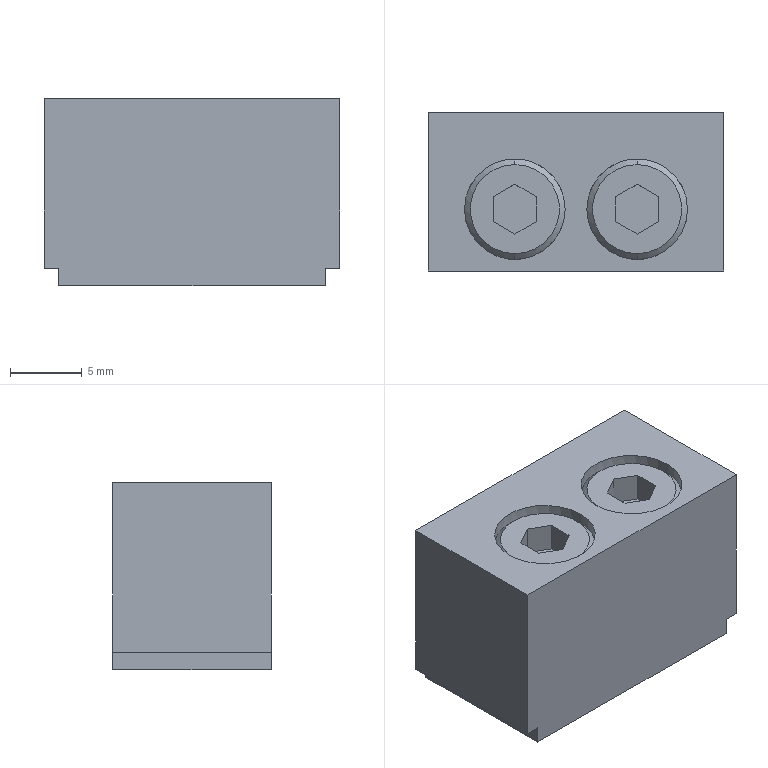Part | SolidWorks | features RefAxis 6, ICE 3, 3DProfileFeature 2, HoleWzd 2, Revolution 2, Extrusion 1 | 1 solid | 34 faces | box 20.5 x 11 x 13 mm | volume 2840 mm3 | plane 26 | cone 4 | cylinder 4 | commonest cylinder face diameters 7 x4
STEP:
#1=CARTESIAN_POINT('',(14.5,1.2,-0.4));
#2=VERTEX_POINT('',#1);
#3=CARTESIAN_POINT('',(14.5,7.4,-0.4));
#4=VERTEX_POINT('',#3);
#5=CARTESIAN_POINT('',(14.5,4.3,-0.4));
#6=DIRECTION('',(0.,0.,1.));
#7=DIRECTION('',(0.,-1.,0.));
#8=AXIS2_PLACEMENT_3D('',#5,#6,#7);
#9=CIRCLE('',#8,3.1);
#10=EDGE_CURVE('',#2,#4,#9,.T.);
#11=ORIENTED_EDGE('',*,*,#10,.F.);
#12=CARTESIAN_POINT('',(14.5,0.8,-0.8));
#13=VERTEX_POINT('',#12);
#14=CARTESIAN_POINT('',(14.5,0.8,-0.8));
#15=DIRECTION('',(0.,-0.7071,-0.7071));
#16=VECTOR('',#15,1000.);
#17=LINE('',#14,#16);
#18=EDGE_CURVE('',#2,#13,#17,.T.);
#19=ORIENTED_EDGE('',*,*,#18,.T.);
#20=CARTESIAN_POINT('',(18.,4.3,-0.8));
#21=VERTEX_POINT('',#20);
#22=CARTESIAN_POINT('',(14.5,4.3,-0.8));
#23=DIRECTION('',(0.,0.,1.));
#24=DIRECTION('',(0.,1.,0.));
#25=AXIS2_PLACEMENT_3D('',#22,#23,#24);
#26=CIRCLE('',#25,3.5);
#27=EDGE_CURVE('',#13,#21,#26,.T.);
#28=ORIENTED_EDGE('',*,*,#27,.T.);
#29=CARTESIAN_POINT('',(14.5,7.8,-0.8));
#30=VERTEX_POINT('',#29);
#31=CARTESIAN_POINT('',(14.5,4.3,-0.8));
#32=DIRECTION('',(0.,0.,1.));
#33=DIRECTION('',(0.,1.,0.));
#34=AXIS2_PLACEMENT_3D('',#31,#32,#33);
#35=CIRCLE('',#34,3.5);
#36=EDGE_CURVE('',#21,#30,#35,.T.);
#37=ORIENTED_EDGE('',*,*,#36,.T.);
#38=CARTESIAN_POINT('',(14.5,7.8,-0.8));
#39=DIRECTION('',(0.,0.7071,-0.7071));
#40=VECTOR('',#39,1000.);
#41=LINE('',#38,#40);
#42=EDGE_CURVE('',#4,#30,#41,.T.);
#43=ORIENTED_EDGE('',*,*,#42,.F.);
#44=EDGE_LOOP('',(#11,#19,#28,#37,#43));
#45=FACE_OUTER_BOUND('',#44,.T.);
#46=CARTESIAN_POINT('',(14.5,4.3,-0.8));
#47=DIRECTION('',(0.,0.,-1.));
#48=DIRECTION('',(0.,1.,0.));
#49=AXIS2_PLACEMENT_3D('',#46,#47,#48);
#50=CONICAL_SURFACE('',#49,3.5,0.7854);
#51=ADVANCED_FACE('',(#45),#50,.T.);
#52=CARTESIAN_POINT('',(6.,1.2,-0.4));
#53=VERTEX_POINT('',#52);
#54=CARTESIAN_POINT('',(6.,7.4,-0.4));
#55=VERTEX_POINT('',#54);
#56=CARTESIAN_POINT('',(6.,4.3,-0.4));
#57=DIRECTION('',(0.,0.,1.));
#58=DIRECTION('',(0.,-1.,0.));
#59=AXIS2_PLACEMENT_3D('',#56,#57,#58);
#60=CIRCLE('',#59,3.1);
#61=EDGE_CURVE('',#53,#55,#60,.T.);
#62=ORIENTED_EDGE('',*,*,#61,.F.);
#63=CARTESIAN_POINT('',(6.,0.8,-0.8));
#64=VERTEX_POINT('',#63);
#65=CARTESIAN_POINT('',(6.,0.8,-0.8));
#66=DIRECTION('',(0.,-0.7071,-0.7071));
#67=VECTOR('',#66,1000.);
#68=LINE('',#65,#67);
#69=EDGE_CURVE('',#53,#64,#68,.T.);
#70=ORIENTED_EDGE('',*,*,#69,.T.);
#71=CARTESIAN_POINT('',(9.5,4.3,-0.8));
#72=VERTEX_POINT('',#71);
#73=CARTESIAN_POINT('',(6.,4.3,-0.8));
#74=DIRECTION('',(0.,0.,1.));
#75=DIRECTION('',(0.,1.,0.));
#76=AXIS2_PLACEMENT_3D('',#73,#74,#75);
#77=CIRCLE('',#76,3.5);
#78=EDGE_CURVE('',#64,#72,#77,.T.);
#79=ORIENTED_EDGE('',*,*,#78,.T.);
#80=CARTESIAN_POINT('',(6.,7.8,-0.8));
#81=VERTEX_POINT('',#80);
#82=CARTESIAN_POINT('',(6.,4.3,-0.8));
#83=DIRECTION('',(0.,0.,1.));
#84=DIRECTION('',(0.,1.,0.));
#85=AXIS2_PLACEMENT_3D('',#82,#83,#84);
#86=CIRCLE('',#85,3.5);
#87=EDGE_CURVE('',#72,#81,#86,.T.);
#88=ORIENTED_EDGE('',*,*,#87,.T.);
#89=CARTESIAN_POINT('',(6.,7.8,-0.8));
#90=DIRECTION('',(0.,0.7071,-0.7071));
#91=VECTOR('',#90,1000.);
#92=LINE('',#89,#91);
#93=EDGE_CURVE('',#55,#81,#92,.T.);
#94=ORIENTED_EDGE('',*,*,#93,.F.);
#95=EDGE_LOOP('',(#62,#70,#79,#88,#94));
#96=FACE_OUTER_BOUND('',#95,.T.);
#97=CARTESIAN_POINT('',(6.,4.3,-0.8));
#98=DIRECTION('',(0.,0.,-1.));
#99=DIRECTION('',(0.,1.,0.));
#100=AXIS2_PLACEMENT_3D('',#97,#98,#99);
#101=CONICAL_SURFACE('',#100,3.5,0.7854);
#102=ADVANCED_FACE('',(#96),#101,.T.);
#103=CARTESIAN_POINT('',(2.5,4.3,-0.8));
#104=VERTEX_POINT('',#103);
#105=CARTESIAN_POINT('',(6.,4.3,-0.8));
#106=DIRECTION('',(0.,0.,1.));
#107=DIRECTION('',(0.,1.,0.));
#108=AXIS2_PLACEMENT_3D('',#105,#106,#107);
#109=CIRCLE('',#108,3.5);
#110=EDGE_CURVE('',#104,#64,#109,.T.);
#111=ORIENTED_EDGE('',*,*,#110,.F.);
#112=CARTESIAN_POINT('',(2.5,4.3,0.));
#113=VERTEX_POINT('',#112);
#114=CARTESIAN_POINT('',(2.5,4.3,0.));
#115=DIRECTION('',(0.,0.,1.));
#116=VECTOR('',#115,1000.);
#117=LINE('',#114,#116);
#118=EDGE_CURVE('',#104,#113,#117,.T.);
#119=ORIENTED_EDGE('',*,*,#118,.T.);
#120=CARTESIAN_POINT('',(9.5,4.3,0.));
#121=VERTEX_POINT('',#120);
#122=CARTESIAN_POINT('',(6.,4.3,0.));
#123=DIRECTION('',(0.,0.,1.));
#124=DIRECTION('',(1.,0.,0.));
#125=AXIS2_PLACEMENT_3D('',#122,#123,#124);
#126=CIRCLE('',#125,3.5);
#127=EDGE_CURVE('',#113,#121,#126,.T.);
#128=ORIENTED_EDGE('',*,*,#127,.T.);
#129=CARTESIAN_POINT('',(9.5,4.3,0.));
#130=DIRECTION('',(0.,0.,1.));
#131=VECTOR('',#130,1000.);
#132=LINE('',#129,#131);
#133=EDGE_CURVE('',#72,#121,#132,.T.);
#134=ORIENTED_EDGE('',*,*,#133,.F.);
#135=ORIENTED_EDGE('',*,*,#78,.F.);
#136=EDGE_LOOP('',(#111,#119,#128,#134,#135));
#137=FACE_OUTER_BOUND('',#136,.T.);
#138=CARTESIAN_POINT('',(6.,4.3,0.));
#139=DIRECTION('',(0.,0.,1.));
#140=DIRECTION('',(1.,0.,0.));
#141=AXIS2_PLACEMENT_3D('',#138,#139,#140);
#142=CYLINDRICAL_SURFACE('',#141,3.5);
#143=ADVANCED_FACE('',(#137),#142,.F.);
#144=CARTESIAN_POINT('',(11.,4.3,-0.8));
#145=VERTEX_POINT('',#144);
#146=CARTESIAN_POINT('',(14.5,4.3,-0.8));
#147=DIRECTION('',(0.,0.,1.));
#148=DIRECTION('',(0.,1.,0.));
#149=AXIS2_PLACEMENT_3D('',#146,#147,#148);
#150=CIRCLE('',#149,3.5);
#151=EDGE_CURVE('',#145,#13,#150,.T.);
#152=ORIENTED_EDGE('',*,*,#151,.F.);
#153=CARTESIAN_POINT('',(11.,4.3,0.));
#154=VERTEX_POINT('',#153);
#155=CARTESIAN_POINT('',(11.,4.3,0.));
#156=DIRECTION('',(0.,0.,1.));
#157=VECTOR('',#156,1000.);
#158=LINE('',#155,#157);
#159=EDGE_CURVE('',#145,#154,#158,.T.);
#160=ORIENTED_EDGE('',*,*,#159,.T.);
#161=CARTESIAN_POINT('',(18.,4.3,0.));
#162=VERTEX_POINT('',#161);
#163=CARTESIAN_POINT('',(14.5,4.3,0.));
#164=DIRECTION('',(0.,0.,1.));
#165=DIRECTION('',(1.,0.,0.));
#166=AXIS2_PLACEMENT_3D('',#163,#164,#165);
#167=CIRCLE('',#166,3.5);
#168=EDGE_CURVE('',#154,#162,#167,.T.);
#169=ORIENTED_EDGE('',*,*,#168,.T.);
#170=CARTESIAN_POINT('',(18.,4.3,0.));
#171=DIRECTION('',(0.,0.,1.));
#172=VECTOR('',#171,1000.);
#173=LINE('',#170,#172);
#174=EDGE_CURVE('',#21,#162,#173,.T.);
#175=ORIENTED_EDGE('',*,*,#174,.F.);
#176=ORIENTED_EDGE('',*,*,#27,.F.);
#177=EDGE_LOOP('',(#152,#160,#169,#175,#176));
#178=FACE_OUTER_BOUND('',#177,.T.);
#179=CARTESIAN_POINT('',(14.5,4.3,0.));
#180=DIRECTION('',(0.,0.,1.));
#181=DIRECTION('',(1.,0.,0.));
#182=AXIS2_PLACEMENT_3D('',#179,#180,#181);
#183=CYLINDRICAL_SURFACE('',#182,3.5);
#184=ADVANCED_FACE('',(#178),#183,.F.);
#185=ORIENTED_EDGE('',*,*,#159,.F.);
#186=CARTESIAN_POINT('',(14.5,4.3,-0.8));
#187=DIRECTION('',(0.,0.,1.));
#188=DIRECTION('',(0.,1.,0.));
#189=AXIS2_PLACEMENT_3D('',#186,#187,#188);
#190=CIRCLE('',#189,3.5);
#191=EDGE_CURVE('',#30,#145,#190,.T.);
#192=ORIENTED_EDGE('',*,*,#191,.F.);
#193=ORIENTED_EDGE('',*,*,#36,.F.);
#194=ORIENTED_EDGE('',*,*,#174,.T.);
#195=CARTESIAN_POINT('',(14.5,4.3,0.));
#196=DIRECTION('',(0.,0.,1.));
#197=DIRECTION('',(1.,0.,0.));
#198=AXIS2_PLACEMENT_3D('',#195,#196,#197);
#199=CIRCLE('',#198,3.5);
#200=EDGE_CURVE('',#162,#154,#199,.T.);
#201=ORIENTED_EDGE('',*,*,#200,.T.);
#202=EDGE_LOOP('',(#185,#192,#193,#194,#201));
#203=FACE_OUTER_BOUND('',#202,.T.);
#204=CARTESIAN_POINT('',(14.5,4.3,0.));
#205=DIRECTION('',(0.,0.,1.));
#206=DIRECTION('',(1.,0.,0.));
#207=AXIS2_PLACEMENT_3D('',#204,#205,#206);
#208=CYLINDRICAL_SURFACE('',#207,3.5);
#209=ADVANCED_FACE('',(#203),#208,.F.);
#210=ORIENTED_EDGE('',*,*,#118,.F.);
#211=CARTESIAN_POINT('',(6.,4.3,-0.8));
#212=DIRECTION('',(0.,0.,1.));
#213=DIRECTION('',(0.,1.,0.));
#214=AXIS2_PLACEMENT_3D('',#211,#212,#213);
#215=CIRCLE('',#214,3.5);
#216=EDGE_CURVE('',#81,#104,#215,.T.);
#217=ORIENTED_EDGE('',*,*,#216,.F.);
#218=ORIENTED_EDGE('',*,*,#87,.F.);
#219=ORIENTED_EDGE('',*,*,#133,.T.);
#220=CARTESIAN_POINT('',(6.,4.3,0.));
#221=DIRECTION('',(0.,0.,1.));
#222=DIRECTION('',(1.,0.,0.));
#223=AXIS2_PLACEMENT_3D('',#220,#221,#222);
#224=CIRCLE('',#223,3.5);
#225=EDGE_CURVE('',#121,#113,#224,.T.);
#226=ORIENTED_EDGE('',*,*,#225,.T.);
#227=EDGE_LOOP('',(#210,#217,#218,#219,#226));
#228=FACE_OUTER_BOUND('',#227,.T.);
#229=CARTESIAN_POINT('',(6.,4.3,0.));
#230=DIRECTION('',(0.,0.,1.));
#231=DIRECTION('',(1.,0.,0.));
#232=AXIS2_PLACEMENT_3D('',#229,#230,#231);
#233=CYLINDRICAL_SURFACE('',#232,3.5);
#234=ADVANCED_FACE('',(#228),#233,.F.);
#235=CARTESIAN_POINT('',(0.,11.,-11.8));
#236=VERTEX_POINT('',#235);
#237=CARTESIAN_POINT('',(0.,0.,-11.8));
#238=VERTEX_POINT('',#237);
#239=CARTESIAN_POINT('',(0.,13.,-11.8));
#240=DIRECTION('',(0.,-1.,0.));
#241=VECTOR('',#240,1000.);
#242=LINE('',#239,#241);
#243=EDGE_CURVE('',#236,#238,#242,.T.);
#244=ORIENTED_EDGE('',*,*,#243,.T.);
#245=CARTESIAN_POINT('',(0.,0.,0.));
#246=VERTEX_POINT('',#245);
#247=CARTESIAN_POINT('',(0.,0.,-13.));
#248=DIRECTION('',(0.,0.,1.));
#249=VECTOR('',#248,1000.);
#250=LINE('',#247,#249);
#251=EDGE_CURVE('',#238,#246,#250,.T.);
#252=ORIENTED_EDGE('',*,*,#251,.T.);
#253=CARTESIAN_POINT('',(0.,11.,0.));
#254=VERTEX_POINT('',#253);
#255=CARTESIAN_POINT('',(0.,11.,0.));
#256=DIRECTION('',(0.,-1.,0.));
#257=VECTOR('',#256,1000.);
#258=LINE('',#255,#257);
#259=EDGE_CURVE('',#254,#246,#258,.T.);
#260=ORIENTED_EDGE('',*,*,#259,.F.);
#261=CARTESIAN_POINT('',(0.,11.,-13.));
#262=DIRECTION('',(0.,0.,1.));
#263=VECTOR('',#262,1000.);
#264=LINE('',#261,#263);
#265=EDGE_CURVE('',#236,#254,#264,.T.);
#266=ORIENTED_EDGE('',*,*,#265,.F.);
#267=EDGE_LOOP('',(#244,#252,#260,#266));
#268=FACE_OUTER_BOUND('',#267,.T.);
#269=CARTESIAN_POINT('',(0.,11.,-13.));
#270=DIRECTION('',(1.,0.,0.));
#271=DIRECTION('',(0.,0.,-1.));
#272=AXIS2_PLACEMENT_3D('',#269,#270,#271);
#273=PLANE('',#272);
#274=ADVANCED_FACE('',(#268),#273,.F.);
#275=CARTESIAN_POINT('',(20.5,11.,-11.8));
#276=VERTEX_POINT('',#275);
#277=CARTESIAN_POINT('',(20.5,0.,-11.8));
#278=VERTEX_POINT('',#277);
#279=CARTESIAN_POINT('',(20.5,13.,-11.8));
#280=DIRECTION('',(0.,-1.,0.));
#281=VECTOR('',#280,1000.);
#282=LINE('',#279,#281);
#283=EDGE_CURVE('',#276,#278,#282,.T.);
#284=ORIENTED_EDGE('',*,*,#283,.F.);
#285=CARTESIAN_POINT('',(20.5,11.,0.));
#286=VERTEX_POINT('',#285);
#287=CARTESIAN_POINT('',(20.5,11.,0.));
#288=DIRECTION('',(0.,0.,-1.));
#289=VECTOR('',#288,1000.);
#290=LINE('',#287,#289);
#291=EDGE_CURVE('',#286,#276,#290,.T.);
#292=ORIENTED_EDGE('',*,*,#291,.F.);
#293=CARTESIAN_POINT('',(20.5,0.,0.));
#294=VERTEX_POINT('',#293);
#295=CARTESIAN_POINT('',(20.5,11.,0.));
#296=DIRECTION('',(0.,-1.,0.));
#297=VECTOR('',#296,1000.);
#298=LINE('',#295,#297);
#299=EDGE_CURVE('',#286,#294,#298,.T.);
#300=ORIENTED_EDGE('',*,*,#299,.T.);
#301=CARTESIAN_POINT('',(20.5,0.,0.));
#302=DIRECTION('',(0.,0.,-1.));
#303=VECTOR('',#302,1000.);
#304=LINE('',#301,#303);
#305=EDGE_CURVE('',#294,#278,#304,.T.);
#306=ORIENTED_EDGE('',*,*,#305,.T.);
#307=EDGE_LOOP('',(#284,#292,#300,#306));
#308=FACE_OUTER_BOUND('',#307,.T.);
#309=CARTESIAN_POINT('',(20.5,11.,0.));
#310=DIRECTION('',(-1.,0.,0.));
#311=DIRECTION('',(0.,0.,1.));
#312=AXIS2_PLACEMENT_3D('',#309,#310,#311);
#313=PLANE('',#312);
#314=ADVANCED_FACE('',(#308),#313,.F.);
#315=CARTESIAN_POINT('',(1.,11.,-13.));
#316=VERTEX_POINT('',#315);
#317=CARTESIAN_POINT('',(1.,0.,-13.));
#318=VERTEX_POINT('',#317);
#319=CARTESIAN_POINT('',(1.,13.,-13.));
#320=DIRECTION('',(0.,-1.,0.));
#321=VECTOR('',#320,1000.);
#322=LINE('',#319,#321);
#323=EDGE_CURVE('',#316,#318,#322,.T.);
#324=ORIENTED_EDGE('',*,*,#323,.F.);
#325=CARTESIAN_POINT('',(19.5,11.,-13.));
#326=VERTEX_POINT('',#325);
#327=CARTESIAN_POINT('',(20.5,11.,-13.));
#328=DIRECTION('',(-1.,0.,0.));
#329=VECTOR('',#328,1000.);
#330=LINE('',#327,#329);
#331=EDGE_CURVE('',#326,#316,#330,.T.);
#332=ORIENTED_EDGE('',*,*,#331,.F.);
#333=CARTESIAN_POINT('',(19.5,0.,-13.));
#334=VERTEX_POINT('',#333);
#335=CARTESIAN_POINT('',(19.5,13.,-13.));
#336=DIRECTION('',(0.,-1.,0.));
#337=VECTOR('',#336,1000.);
#338=LINE('',#335,#337);
#339=EDGE_CURVE('',#326,#334,#338,.T.);
#340=ORIENTED_EDGE('',*,*,#339,.T.);
#341=CARTESIAN_POINT('',(20.5,0.,-13.));
#342=DIRECTION('',(-1.,0.,0.));
#343=VECTOR('',#342,1000.);
#344=LINE('',#341,#343);
#345=EDGE_CURVE('',#334,#318,#344,.T.);
#346=ORIENTED_EDGE('',*,*,#345,.T.);
#347=EDGE_LOOP('',(#324,#332,#340,#346));
#348=FACE_OUTER_BOUND('',#347,.T.);
#349=CARTESIAN_POINT('',(20.5,11.,-13.));
#350=DIRECTION('',(0.,0.,1.));
#351=DIRECTION('',(1.,0.,0.));
#352=AXIS2_PLACEMENT_3D('',#349,#350,#351);
#353=PLANE('',#352);
#354=ADVANCED_FACE('',(#348),#353,.F.);
#355=CARTESIAN_POINT('',(1.,11.,-11.8));
#356=VERTEX_POINT('',#355);
#357=CARTESIAN_POINT('',(1.,11.,0.));
#358=DIRECTION('',(0.,0.,1.));
#359=VECTOR('',#358,1000.);
#360=LINE('',#357,#359);
#361=EDGE_CURVE('',#316,#356,#360,.T.);
#362=ORIENTED_EDGE('',*,*,#361,.T.);
#363=CARTESIAN_POINT('',(0.,11.,-11.8));
#364=DIRECTION('',(-1.,0.,0.));
#365=VECTOR('',#364,1000.);
#366=LINE('',#363,#365);
#367=EDGE_CURVE('',#356,#236,#366,.T.);
#368=ORIENTED_EDGE('',*,*,#367,.T.);
#369=ORIENTED_EDGE('',*,*,#265,.T.);
#370=CARTESIAN_POINT('',(0.,11.,0.));
#371=DIRECTION('',(1.,0.,0.));
#372=VECTOR('',#371,1000.);
#373=LINE('',#370,#372);
#374=EDGE_CURVE('',#254,#286,#373,.T.);
#375=ORIENTED_EDGE('',*,*,#374,.T.);
#376=ORIENTED_EDGE('',*,*,#291,.T.);
#377=CARTESIAN_POINT('',(19.5,11.,-11.8));
#378=VERTEX_POINT('',#377);
#379=CARTESIAN_POINT('',(0.,11.,-11.8));
#380=DIRECTION('',(-1.,0.,0.));
#381=VECTOR('',#380,1000.);
#382=LINE('',#379,#381);
#383=EDGE_CURVE('',#276,#378,#382,.T.);
#384=ORIENTED_EDGE('',*,*,#383,.T.);
#385=CARTESIAN_POINT('',(19.5,11.,0.));
#386=DIRECTION('',(0.,0.,-1.));
#387=VECTOR('',#386,1000.);
#388=LINE('',#385,#387);
#389=EDGE_CURVE('',#378,#326,#388,.T.);
#390=ORIENTED_EDGE('',*,*,#389,.T.);
#391=ORIENTED_EDGE('',*,*,#331,.T.);
#392=EDGE_LOOP('',(#362,#368,#369,#375,#376,#384,#390,#391));
#393=FACE_OUTER_BOUND('',#392,.T.);
#394=CARTESIAN_POINT('',(0.,11.,0.));
#395=DIRECTION('',(0.,1.,0.));
#396=DIRECTION('',(0.,0.,1.));
#397=AXIS2_PLACEMENT_3D('',#394,#395,#396);
#398=PLANE('',#397);
#399=ADVANCED_FACE('',(#393),#398,.T.);
#400=CARTESIAN_POINT('',(1.,0.,-11.8));
#401=VERTEX_POINT('',#400);
#402=CARTESIAN_POINT('',(0.,0.,-11.8));
#403=DIRECTION('',(1.,0.,0.));
#404=VECTOR('',#403,1000.);
#405=LINE('',#402,#404);
#406=EDGE_CURVE('',#238,#401,#405,.T.);
#407=ORIENTED_EDGE('',*,*,#406,.T.);
#408=CARTESIAN_POINT('',(1.,0.,-11.8));
#409=DIRECTION('',(0.,0.,-1.));
#410=VECTOR('',#409,1000.);
#411=LINE('',#408,#410);
#412=EDGE_CURVE('',#401,#318,#411,.T.);
#413=ORIENTED_EDGE('',*,*,#412,.T.);
#414=ORIENTED_EDGE('',*,*,#345,.F.);
#415=CARTESIAN_POINT('',(19.5,0.,-11.8));
#416=VERTEX_POINT('',#415);
#417=CARTESIAN_POINT('',(19.5,0.,-13.));
#418=DIRECTION('',(0.,0.,1.));
#419=VECTOR('',#418,1000.);
#420=LINE('',#417,#419);
#421=EDGE_CURVE('',#334,#416,#420,.T.);
#422=ORIENTED_EDGE('',*,*,#421,.T.);
#423=CARTESIAN_POINT('',(19.5,0.,-11.8));
#424=DIRECTION('',(1.,0.,0.));
#425=VECTOR('',#424,1000.);
#426=LINE('',#423,#425);
#427=EDGE_CURVE('',#416,#278,#426,.T.);
#428=ORIENTED_EDGE('',*,*,#427,.T.);
#429=ORIENTED_EDGE('',*,*,#305,.F.);
#430=CARTESIAN_POINT('',(0.,0.,0.));
#431=DIRECTION('',(1.,0.,0.));
#432=VECTOR('',#431,1000.);
#433=LINE('',#430,#432);
#434=EDGE_CURVE('',#246,#294,#433,.T.);
#435=ORIENTED_EDGE('',*,*,#434,.F.);
#436=ORIENTED_EDGE('',*,*,#251,.F.);
#437=EDGE_LOOP('',(#407,#413,#414,#422,#428,#429,#435,#436));
#438=FACE_OUTER_BOUND('',#437,.T.);
#439=CARTESIAN_POINT('',(0.,0.,0.));
#440=DIRECTION('',(0.,1.,0.));
#441=DIRECTION('',(0.,0.,1.));
#442=AXIS2_PLACEMENT_3D('',#439,#440,#441);
#443=PLANE('',#442);
#444=ADVANCED_FACE('',(#438),#443,.F.);
#445=ORIENTED_EDGE('',*,*,#200,.F.);
#446=ORIENTED_EDGE('',*,*,#168,.F.);
#447=EDGE_LOOP('',(#445,#446));
#448=FACE_BOUND('',#447,.T.);
#449=ORIENTED_EDGE('',*,*,#225,.F.);
#450=ORIENTED_EDGE('',*,*,#127,.F.);
#451=EDGE_LOOP('',(#449,#450));
#452=FACE_BOUND('',#451,.T.);
#453=ORIENTED_EDGE('',*,*,#434,.T.);
#454=ORIENTED_EDGE('',*,*,#299,.F.);
#455=ORIENTED_EDGE('',*,*,#374,.F.);
#456=ORIENTED_EDGE('',*,*,#259,.T.);
#457=EDGE_LOOP('',(#453,#454,#455,#456));
#458=FACE_OUTER_BOUND('',#457,.T.);
#459=CARTESIAN_POINT('',(0.,11.,0.));
#460=DIRECTION('',(0.,0.,-1.));
#461=DIRECTION('',(-1.,0.,0.));
#462=AXIS2_PLACEMENT_3D('',#459,#460,#461);
#463=PLANE('',#462);
#464=ADVANCED_FACE('',(#448,#452,#458),#463,.F.);
#465=ORIENTED_EDGE('',*,*,#283,.T.);
#466=ORIENTED_EDGE('',*,*,#427,.F.);
#467=CARTESIAN_POINT('',(19.5,13.,-11.8));
#468=DIRECTION('',(0.,-1.,0.));
#469=VECTOR('',#468,1000.);
#470=LINE('',#467,#469);
#471=EDGE_CURVE('',#378,#416,#470,.T.);
#472=ORIENTED_EDGE('',*,*,#471,.F.);
#473=ORIENTED_EDGE('',*,*,#383,.F.);
#474=EDGE_LOOP('',(#465,#466,#472,#473));
#475=FACE_OUTER_BOUND('',#474,.T.);
#476=CARTESIAN_POINT('',(19.5,13.,-11.8));
#477=DIRECTION('',(0.,0.,-1.));
#478=DIRECTION('',(-1.,0.,0.));
#479=AXIS2_PLACEMENT_3D('',#476,#477,#478);
#480=PLANE('',#479);
#481=ADVANCED_FACE('',(#475),#480,.T.);
#482=ORIENTED_EDGE('',*,*,#471,.T.);
#483=ORIENTED_EDGE('',*,*,#421,.F.);
#484=ORIENTED_EDGE('',*,*,#339,.F.);
#485=ORIENTED_EDGE('',*,*,#389,.F.);
#486=EDGE_LOOP('',(#482,#483,#484,#485));
#487=FACE_OUTER_BOUND('',#486,.T.);
#488=CARTESIAN_POINT('',(19.5,13.,-13.));
#489=DIRECTION('',(1.,0.,0.));
#490=DIRECTION('',(0.,0.,-1.));
#491=AXIS2_PLACEMENT_3D('',#488,#489,#490);
#492=PLANE('',#491);
#493=ADVANCED_FACE('',(#487),#492,.T.);
#494=CARTESIAN_POINT('',(1.,13.,-11.8));
#495=DIRECTION('',(0.,-1.,0.));
#496=VECTOR('',#495,1000.);
#497=LINE('',#494,#496);
#498=EDGE_CURVE('',#356,#401,#497,.T.);
#499=ORIENTED_EDGE('',*,*,#498,.T.);
#500=ORIENTED_EDGE('',*,*,#406,.F.);
#501=ORIENTED_EDGE('',*,*,#243,.F.);
#502=ORIENTED_EDGE('',*,*,#367,.F.);
#503=EDGE_LOOP('',(#499,#500,#501,#502));
#504=FACE_OUTER_BOUND('',#503,.T.);
#505=CARTESIAN_POINT('',(0.,13.,-11.8));
#506=DIRECTION('',(0.,0.,-1.));
#507=DIRECTION('',(-1.,0.,0.));
#508=AXIS2_PLACEMENT_3D('',#505,#506,#507);
#509=PLANE('',#508);
#510=ADVANCED_FACE('',(#504),#509,.T.);
#511=ORIENTED_EDGE('',*,*,#323,.T.);
#512=ORIENTED_EDGE('',*,*,#412,.F.);
#513=ORIENTED_EDGE('',*,*,#498,.F.);
#514=ORIENTED_EDGE('',*,*,#361,.F.);
#515=EDGE_LOOP('',(#511,#512,#513,#514));
#516=FACE_OUTER_BOUND('',#515,.T.);
#517=CARTESIAN_POINT('',(1.,13.,-11.8));
#518=DIRECTION('',(-1.,0.,0.));
#519=DIRECTION('',(0.,0.,1.));
#520=AXIS2_PLACEMENT_3D('',#517,#518,#519);
#521=PLANE('',#520);
#522=ADVANCED_FACE('',(#516),#521,.T.);
#523=CARTESIAN_POINT('',(4.5,5.166,-0.4));
#524=VERTEX_POINT('',#523);
#525=CARTESIAN_POINT('',(4.5,3.434,-0.4));
#526=VERTEX_POINT('',#525);
#527=CARTESIAN_POINT('',(4.5,5.166,-0.4));
#528=DIRECTION('',(0.,-1.,0.));
#529=VECTOR('',#528,1000.);
#530=LINE('',#527,#529);
#531=EDGE_CURVE('',#524,#526,#530,.T.);
#532=ORIENTED_EDGE('',*,*,#531,.F.);
#533=CARTESIAN_POINT('',(6.,6.032,-0.4));
#534=VERTEX_POINT('',#533);
#535=CARTESIAN_POINT('',(6.,6.032,-0.4));
#536=DIRECTION('',(-0.866,-0.5,0.));
#537=VECTOR('',#536,1000.);
#538=LINE('',#535,#537);
#539=EDGE_CURVE('',#534,#524,#538,.T.);
#540=ORIENTED_EDGE('',*,*,#539,.F.);
#541=CARTESIAN_POINT('',(7.5,5.166,-0.4));
#542=VERTEX_POINT('',#541);
#543=CARTESIAN_POINT('',(7.5,5.166,-0.4));
#544=DIRECTION('',(-0.866,0.5,0.));
#545=VECTOR('',#544,1000.);
#546=LINE('',#543,#545);
#547=EDGE_CURVE('',#542,#534,#546,.T.);
#548=ORIENTED_EDGE('',*,*,#547,.F.);
#549=CARTESIAN_POINT('',(7.5,3.434,-0.4));
#550=VERTEX_POINT('',#549);
#551=CARTESIAN_POINT('',(7.5,3.434,-0.4));
#552=DIRECTION('',(0.,1.,0.));
#553=VECTOR('',#552,1000.);
#554=LINE('',#551,#553);
#555=EDGE_CURVE('',#550,#542,#554,.T.);
#556=ORIENTED_EDGE('',*,*,#555,.F.);
#557=CARTESIAN_POINT('',(6.,2.568,-0.4));
#558=VERTEX_POINT('',#557);
#559=CARTESIAN_POINT('',(6.,2.568,-0.4));
#560=DIRECTION('',(0.866,0.5,0.));
#561=VECTOR('',#560,1000.);
#562=LINE('',#559,#561);
#563=EDGE_CURVE('',#558,#550,#562,.T.);
#564=ORIENTED_EDGE('',*,*,#563,.F.);
#565=CARTESIAN_POINT('',(4.5,3.434,-0.4));
#566=DIRECTION('',(0.866,-0.5,0.));
#567=VECTOR('',#566,1000.);
#568=LINE('',#565,#567);
#569=EDGE_CURVE('',#526,#558,#568,.T.);
#570=ORIENTED_EDGE('',*,*,#569,.F.);
#571=EDGE_LOOP('',(#532,#540,#548,#556,#564,#570));
#572=FACE_BOUND('',#571,.T.);
#573=CARTESIAN_POINT('',(6.,4.3,-0.4));
#574=DIRECTION('',(0.,0.,1.));
#575=DIRECTION('',(0.,-1.,0.));
#576=AXIS2_PLACEMENT_3D('',#573,#574,#575);
#577=CIRCLE('',#576,3.1);
#578=EDGE_CURVE('',#55,#53,#577,.T.);
#579=ORIENTED_EDGE('',*,*,#578,.T.);
#580=ORIENTED_EDGE('',*,*,#61,.T.);
#581=EDGE_LOOP('',(#579,#580));
#582=FACE_OUTER_BOUND('',#581,.T.);
#583=CARTESIAN_POINT('',(6.,4.3,-0.4));
#584=DIRECTION('',(0.,0.,-1.));
#585=DIRECTION('',(0.,1.,0.));
#586=AXIS2_PLACEMENT_3D('',#583,#584,#585);
#587=PLANE('',#586);
#588=ADVANCED_FACE('',(#572,#582),#587,.F.);
#589=ORIENTED_EDGE('',*,*,#69,.F.);
#590=ORIENTED_EDGE('',*,*,#578,.F.);
#591=ORIENTED_EDGE('',*,*,#93,.T.);
#592=ORIENTED_EDGE('',*,*,#216,.T.);
#593=ORIENTED_EDGE('',*,*,#110,.T.);
#594=EDGE_LOOP('',(#589,#590,#591,#592,#593));
#595=FACE_OUTER_BOUND('',#594,.T.);
#596=CARTESIAN_POINT('',(6.,4.3,-0.8));
#597=DIRECTION('',(0.,0.,-1.));
#598=DIRECTION('',(0.,1.,0.));
#599=AXIS2_PLACEMENT_3D('',#596,#597,#598);
#600=CONICAL_SURFACE('',#599,3.5,0.7854);
#601=ADVANCED_FACE('',(#595),#600,.T.);
#602=CARTESIAN_POINT('',(13.,3.434,-0.4));
#603=VERTEX_POINT('',#602);
#604=CARTESIAN_POINT('',(14.5,2.568,-0.4));
#605=VERTEX_POINT('',#604);
#606=CARTESIAN_POINT('',(13.,3.434,-0.4));
#607=DIRECTION('',(0.866,-0.5,0.));
#608=VECTOR('',#607,1000.);
#609=LINE('',#606,#608);
#610=EDGE_CURVE('',#603,#605,#609,.T.);
#611=ORIENTED_EDGE('',*,*,#610,.F.);
#612=CARTESIAN_POINT('',(13.,5.166,-0.4));
#613=VERTEX_POINT('',#612);
#614=CARTESIAN_POINT('',(13.,5.166,-0.4));
#615=DIRECTION('',(0.,-1.,0.));
#616=VECTOR('',#615,1000.);
#617=LINE('',#614,#616);
#618=EDGE_CURVE('',#613,#603,#617,.T.);
#619=ORIENTED_EDGE('',*,*,#618,.F.);
#620=CARTESIAN_POINT('',(14.5,6.032,-0.4));
#621=VERTEX_POINT('',#620);
#622=CARTESIAN_POINT('',(14.5,6.032,-0.4));
#623=DIRECTION('',(-0.866,-0.5,0.));
#624=VECTOR('',#623,1000.);
#625=LINE('',#622,#624);
#626=EDGE_CURVE('',#621,#613,#625,.T.);
#627=ORIENTED_EDGE('',*,*,#626,.F.);
#628=CARTESIAN_POINT('',(16.,5.166,-0.4));
#629=VERTEX_POINT('',#628);
#630=CARTESIAN_POINT('',(16.,5.166,-0.4));
#631=DIRECTION('',(-0.866,0.5,0.));
#632=VECTOR('',#631,1000.);
#633=LINE('',#630,#632);
#634=EDGE_CURVE('',#629,#621,#633,.T.);
#635=ORIENTED_EDGE('',*,*,#634,.F.);
#636=CARTESIAN_POINT('',(16.,3.434,-0.4));
#637=VERTEX_POINT('',#636);
#638=CARTESIAN_POINT('',(16.,3.434,-0.4));
#639=DIRECTION('',(0.,1.,0.));
#640=VECTOR('',#639,1000.);
#641=LINE('',#638,#640);
#642=EDGE_CURVE('',#637,#629,#641,.T.);
#643=ORIENTED_EDGE('',*,*,#642,.F.);
#644=CARTESIAN_POINT('',(14.5,2.568,-0.4));
#645=DIRECTION('',(0.866,0.5,0.));
#646=VECTOR('',#645,1000.);
#647=LINE('',#644,#646);
#648=EDGE_CURVE('',#605,#637,#647,.T.);
#649=ORIENTED_EDGE('',*,*,#648,.F.);
#650=EDGE_LOOP('',(#611,#619,#627,#635,#643,#649));
#651=FACE_BOUND('',#650,.T.);
#652=CARTESIAN_POINT('',(14.5,4.3,-0.4));
#653=DIRECTION('',(0.,0.,1.));
#654=DIRECTION('',(0.,-1.,0.));
#655=AXIS2_PLACEMENT_3D('',#652,#653,#654);
#656=CIRCLE('',#655,3.1);
#657=EDGE_CURVE('',#4,#2,#656,.T.);
#658=ORIENTED_EDGE('',*,*,#657,.T.);
#659=ORIENTED_EDGE('',*,*,#10,.T.);
#660=EDGE_LOOP('',(#658,#659));
#661=FACE_OUTER_BOUND('',#660,.T.);
#662=CARTESIAN_POINT('',(14.5,4.3,-0.4));
#663=DIRECTION('',(0.,0.,-1.));
#664=DIRECTION('',(0.,1.,0.));
#665=AXIS2_PLACEMENT_3D('',#662,#663,#664);
#666=PLANE('',#665);
#667=ADVANCED_FACE('',(#651,#661),#666,.F.);
#668=ORIENTED_EDGE('',*,*,#18,.F.);
#669=ORIENTED_EDGE('',*,*,#657,.F.);
#670=ORIENTED_EDGE('',*,*,#42,.T.);
#671=ORIENTED_EDGE('',*,*,#191,.T.);
#672=ORIENTED_EDGE('',*,*,#151,.T.);
#673=EDGE_LOOP('',(#668,#669,#670,#671,#672));
#674=FACE_OUTER_BOUND('',#673,.T.);
#675=CARTESIAN_POINT('',(14.5,4.3,-0.8));
#676=DIRECTION('',(0.,0.,-1.));
#677=DIRECTION('',(0.,1.,0.));
#678=AXIS2_PLACEMENT_3D('',#675,#676,#677);
#679=CONICAL_SURFACE('',#678,3.5,0.7854);
#680=ADVANCED_FACE('',(#674),#679,.T.);
#681=ORIENTED_EDGE('',*,*,#539,.T.);
#682=CARTESIAN_POINT('',(4.5,5.166,-2.4));
#683=VERTEX_POINT('',#682);
#684=CARTESIAN_POINT('',(4.5,5.166,-2.4));
#685=DIRECTION('',(0.,0.,1.));
#686=VECTOR('',#685,1000.);
#687=LINE('',#684,#686);
#688=EDGE_CURVE('',#683,#524,#687,.T.);
#689=ORIENTED_EDGE('',*,*,#688,.F.);
#690=CARTESIAN_POINT('',(6.,6.032,-2.4));
#691=VERTEX_POINT('',#690);
#692=CARTESIAN_POINT('',(6.,6.032,-2.4));
#693=DIRECTION('',(-0.866,-0.5,0.));
#694=VECTOR('',#693,1000.);
#695=LINE('',#692,#694);
#696=EDGE_CURVE('',#691,#683,#695,.T.);
#697=ORIENTED_EDGE('',*,*,#696,.F.);
#698=CARTESIAN_POINT('',(6.,6.032,-2.4));
#699=DIRECTION('',(0.,0.,1.));
#700=VECTOR('',#699,1000.);
#701=LINE('',#698,#700);
#702=EDGE_CURVE('',#691,#534,#701,.T.);
#703=ORIENTED_EDGE('',*,*,#702,.T.);
#704=EDGE_LOOP('',(#681,#689,#697,#703));
#705=FACE_OUTER_BOUND('',#704,.T.);
#706=CARTESIAN_POINT('',(6.,6.032,-2.4));
#707=DIRECTION('',(-0.5,0.866,0.));
#708=DIRECTION('',(-0.866,-0.5,0.));
#709=AXIS2_PLACEMENT_3D('',#706,#707,#708);
#710=PLANE('',#709);
#711=ADVANCED_FACE('',(#705),#710,.F.);
#712=ORIENTED_EDGE('',*,*,#547,.T.);
#713=ORIENTED_EDGE('',*,*,#702,.F.);
#714=CARTESIAN_POINT('',(7.5,5.166,-2.4));
#715=VERTEX_POINT('',#714);
#716=CARTESIAN_POINT('',(7.5,5.166,-2.4));
#717=DIRECTION('',(-0.866,0.5,0.));
#718=VECTOR('',#717,1000.);
#719=LINE('',#716,#718);
#720=EDGE_CURVE('',#715,#691,#719,.T.);
#721=ORIENTED_EDGE('',*,*,#720,.F.);
#722=CARTESIAN_POINT('',(7.5,5.166,-2.4));
#723=DIRECTION('',(0.,0.,1.));
#724=VECTOR('',#723,1000.);
#725=LINE('',#722,#724);
#726=EDGE_CURVE('',#715,#542,#725,.T.);
#727=ORIENTED_EDGE('',*,*,#726,.T.);
#728=EDGE_LOOP('',(#712,#713,#721,#727));
#729=FACE_OUTER_BOUND('',#728,.T.);
#730=CARTESIAN_POINT('',(7.5,5.166,-2.4));
#731=DIRECTION('',(0.5,0.866,0.));
#732=DIRECTION('',(-0.866,0.5,0.));
#733=AXIS2_PLACEMENT_3D('',#730,#731,#732);
#734=PLANE('',#733);
#735=ADVANCED_FACE('',(#729),#734,.F.);
#736=ORIENTED_EDGE('',*,*,#555,.T.);
#737=ORIENTED_EDGE('',*,*,#726,.F.);
#738=CARTESIAN_POINT('',(7.5,3.434,-2.4));
#739=VERTEX_POINT('',#738);
#740=CARTESIAN_POINT('',(7.5,3.434,-2.4));
#741=DIRECTION('',(0.,1.,0.));
#742=VECTOR('',#741,1000.);
#743=LINE('',#740,#742);
#744=EDGE_CURVE('',#739,#715,#743,.T.);
#745=ORIENTED_EDGE('',*,*,#744,.F.);
#746=CARTESIAN_POINT('',(7.5,3.434,-2.4));
#747=DIRECTION('',(0.,0.,1.));
#748=VECTOR('',#747,1000.);
#749=LINE('',#746,#748);
#750=EDGE_CURVE('',#739,#550,#749,.T.);
#751=ORIENTED_EDGE('',*,*,#750,.T.);
#752=EDGE_LOOP('',(#736,#737,#745,#751));
#753=FACE_OUTER_BOUND('',#752,.T.);
#754=CARTESIAN_POINT('',(7.5,3.434,-2.4));
#755=DIRECTION('',(1.,0.,0.));
#756=DIRECTION('',(0.,0.,-1.));
#757=AXIS2_PLACEMENT_3D('',#754,#755,#756);
#758=PLANE('',#757);
#759=ADVANCED_FACE('',(#753),#758,.F.);
#760=ORIENTED_EDGE('',*,*,#563,.T.);
#761=ORIENTED_EDGE('',*,*,#750,.F.);
#762=CARTESIAN_POINT('',(6.,2.568,-2.4));
#763=VERTEX_POINT('',#762);
#764=CARTESIAN_POINT('',(6.,2.568,-2.4));
#765=DIRECTION('',(0.866,0.5,0.));
#766=VECTOR('',#765,1000.);
#767=LINE('',#764,#766);
#768=EDGE_CURVE('',#763,#739,#767,.T.);
#769=ORIENTED_EDGE('',*,*,#768,.F.);
#770=CARTESIAN_POINT('',(6.,2.568,-2.4));
#771=DIRECTION('',(0.,0.,1.));
#772=VECTOR('',#771,1000.);
#773=LINE('',#770,#772);
#774=EDGE_CURVE('',#763,#558,#773,.T.);
#775=ORIENTED_EDGE('',*,*,#774,.T.);
#776=EDGE_LOOP('',(#760,#761,#769,#775));
#777=FACE_OUTER_BOUND('',#776,.T.);
#778=CARTESIAN_POINT('',(6.,2.568,-2.4));
#779=DIRECTION('',(0.5,-0.866,0.));
#780=DIRECTION('',(0.866,0.5,0.));
#781=AXIS2_PLACEMENT_3D('',#778,#779,#780);
#782=PLANE('',#781);
#783=ADVANCED_FACE('',(#777),#782,.F.);
#784=ORIENTED_EDGE('',*,*,#569,.T.);
#785=ORIENTED_EDGE('',*,*,#774,.F.);
#786=CARTESIAN_POINT('',(4.5,3.434,-2.4));
#787=VERTEX_POINT('',#786);
#788=CARTESIAN_POINT('',(4.5,3.434,-2.4));
#789=DIRECTION('',(0.866,-0.5,0.));
#790=VECTOR('',#789,1000.);
#791=LINE('',#788,#790);
#792=EDGE_CURVE('',#787,#763,#791,.T.);
#793=ORIENTED_EDGE('',*,*,#792,.F.);
#794=CARTESIAN_POINT('',(4.5,3.434,-2.4));
#795=DIRECTION('',(0.,0.,1.));
#796=VECTOR('',#795,1000.);
#797=LINE('',#794,#796);
#798=EDGE_CURVE('',#787,#526,#797,.T.);
#799=ORIENTED_EDGE('',*,*,#798,.T.);
#800=EDGE_LOOP('',(#784,#785,#793,#799));
#801=FACE_OUTER_BOUND('',#800,.T.);
#802=CARTESIAN_POINT('',(4.5,3.434,-2.4));
#803=DIRECTION('',(-0.5,-0.866,0.));
#804=DIRECTION('',(0.866,-0.5,0.));
#805=AXIS2_PLACEMENT_3D('',#802,#803,#804);
#806=PLANE('',#805);
#807=ADVANCED_FACE('',(#801),#806,.F.);
#808=ORIENTED_EDGE('',*,*,#531,.T.);
#809=ORIENTED_EDGE('',*,*,#798,.F.);
#810=CARTESIAN_POINT('',(4.5,5.166,-2.4));
#811=DIRECTION('',(0.,-1.,0.));
#812=VECTOR('',#811,1000.);
#813=LINE('',#810,#812);
#814=EDGE_CURVE('',#683,#787,#813,.T.);
#815=ORIENTED_EDGE('',*,*,#814,.F.);
#816=ORIENTED_EDGE('',*,*,#688,.T.);
#817=EDGE_LOOP('',(#808,#809,#815,#816));
#818=FACE_OUTER_BOUND('',#817,.T.);
#819=CARTESIAN_POINT('',(4.5,5.166,-2.4));
#820=DIRECTION('',(-1.,0.,0.));
#821=DIRECTION('',(0.,0.,1.));
#822=AXIS2_PLACEMENT_3D('',#819,#820,#821);
#823=PLANE('',#822);
#824=ADVANCED_FACE('',(#818),#823,.F.);
#825=ORIENTED_EDGE('',*,*,#696,.T.);
#826=ORIENTED_EDGE('',*,*,#814,.T.);
#827=ORIENTED_EDGE('',*,*,#792,.T.);
#828=ORIENTED_EDGE('',*,*,#768,.T.);
#829=ORIENTED_EDGE('',*,*,#744,.T.);
#830=ORIENTED_EDGE('',*,*,#720,.T.);
#831=EDGE_LOOP('',(#825,#826,#827,#828,#829,#830));
#832=FACE_OUTER_BOUND('',#831,.T.);
#833=CARTESIAN_POINT('',(0.,0.,-2.4));
#834=DIRECTION('',(0.,0.,1.));
#835=DIRECTION('',(1.,0.,0.));
#836=AXIS2_PLACEMENT_3D('',#833,#834,#835);
#837=PLANE('',#836);
#838=ADVANCED_FACE('',(#832),#837,.T.);
#839=ORIENTED_EDGE('',*,*,#618,.T.);
#840=CARTESIAN_POINT('',(13.,3.434,-2.4));
#841=VERTEX_POINT('',#840);
#842=CARTESIAN_POINT('',(13.,3.434,-2.4));
#843=DIRECTION('',(0.,0.,1.));
#844=VECTOR('',#843,1000.);
#845=LINE('',#842,#844);
#846=EDGE_CURVE('',#841,#603,#845,.T.);
#847=ORIENTED_EDGE('',*,*,#846,.F.);
#848=CARTESIAN_POINT('',(13.,5.166,-2.4));
#849=VERTEX_POINT('',#848);
#850=CARTESIAN_POINT('',(13.,5.166,-2.4));
#851=DIRECTION('',(0.,-1.,0.));
#852=VECTOR('',#851,1000.);
#853=LINE('',#850,#852);
#854=EDGE_CURVE('',#849,#841,#853,.T.);
#855=ORIENTED_EDGE('',*,*,#854,.F.);
#856=CARTESIAN_POINT('',(13.,5.166,-2.4));
#857=DIRECTION('',(0.,0.,1.));
#858=VECTOR('',#857,1000.);
#859=LINE('',#856,#858);
#860=EDGE_CURVE('',#849,#613,#859,.T.);
#861=ORIENTED_EDGE('',*,*,#860,.T.);
#862=EDGE_LOOP('',(#839,#847,#855,#861));
#863=FACE_OUTER_BOUND('',#862,.T.);
#864=CARTESIAN_POINT('',(13.,5.166,-2.4));
#865=DIRECTION('',(-1.,0.,0.));
#866=DIRECTION('',(0.,0.,1.));
#867=AXIS2_PLACEMENT_3D('',#864,#865,#866);
#868=PLANE('',#867);
#869=ADVANCED_FACE('',(#863),#868,.F.);
#870=ORIENTED_EDGE('',*,*,#626,.T.);
#871=ORIENTED_EDGE('',*,*,#860,.F.);
#872=CARTESIAN_POINT('',(14.5,6.032,-2.4));
#873=VERTEX_POINT('',#872);
#874=CARTESIAN_POINT('',(14.5,6.032,-2.4));
#875=DIRECTION('',(-0.866,-0.5,0.));
#876=VECTOR('',#875,1000.);
#877=LINE('',#874,#876);
#878=EDGE_CURVE('',#873,#849,#877,.T.);
#879=ORIENTED_EDGE('',*,*,#878,.F.);
#880=CARTESIAN_POINT('',(14.5,6.032,-2.4));
#881=DIRECTION('',(0.,0.,1.));
#882=VECTOR('',#881,1000.);
#883=LINE('',#880,#882);
#884=EDGE_CURVE('',#873,#621,#883,.T.);
#885=ORIENTED_EDGE('',*,*,#884,.T.);
#886=EDGE_LOOP('',(#870,#871,#879,#885));
#887=FACE_OUTER_BOUND('',#886,.T.);
#888=CARTESIAN_POINT('',(14.5,6.032,-2.4));
#889=DIRECTION('',(-0.5,0.866,0.));
#890=DIRECTION('',(-0.866,-0.5,0.));
#891=AXIS2_PLACEMENT_3D('',#888,#889,#890);
#892=PLANE('',#891);
#893=ADVANCED_FACE('',(#887),#892,.F.);
#894=ORIENTED_EDGE('',*,*,#634,.T.);
#895=ORIENTED_EDGE('',*,*,#884,.F.);
#896=CARTESIAN_POINT('',(16.,5.166,-2.4));
#897=VERTEX_POINT('',#896);
#898=CARTESIAN_POINT('',(16.,5.166,-2.4));
#899=DIRECTION('',(-0.866,0.5,0.));
#900=VECTOR('',#899,1000.);
#901=LINE('',#898,#900);
#902=EDGE_CURVE('',#897,#873,#901,.T.);
#903=ORIENTED_EDGE('',*,*,#902,.F.);
#904=CARTESIAN_POINT('',(16.,5.166,-2.4));
#905=DIRECTION('',(0.,0.,1.));
#906=VECTOR('',#905,1000.);
#907=LINE('',#904,#906);
#908=EDGE_CURVE('',#897,#629,#907,.T.);
#909=ORIENTED_EDGE('',*,*,#908,.T.);
#910=EDGE_LOOP('',(#894,#895,#903,#909));
#911=FACE_OUTER_BOUND('',#910,.T.);
#912=CARTESIAN_POINT('',(16.,5.166,-2.4));
#913=DIRECTION('',(0.5,0.866,0.));
#914=DIRECTION('',(-0.866,0.5,0.));
#915=AXIS2_PLACEMENT_3D('',#912,#913,#914);
#916=PLANE('',#915);
#917=ADVANCED_FACE('',(#911),#916,.F.);
#918=ORIENTED_EDGE('',*,*,#642,.T.);
#919=ORIENTED_EDGE('',*,*,#908,.F.);
#920=CARTESIAN_POINT('',(16.,3.434,-2.4));
#921=VERTEX_POINT('',#920);
#922=CARTESIAN_POINT('',(16.,3.434,-2.4));
#923=DIRECTION('',(0.,1.,0.));
#924=VECTOR('',#923,1000.);
#925=LINE('',#922,#924);
#926=EDGE_CURVE('',#921,#897,#925,.T.);
#927=ORIENTED_EDGE('',*,*,#926,.F.);
#928=CARTESIAN_POINT('',(16.,3.434,-2.4));
#929=DIRECTION('',(0.,0.,1.));
#930=VECTOR('',#929,1000.);
#931=LINE('',#928,#930);
#932=EDGE_CURVE('',#921,#637,#931,.T.);
#933=ORIENTED_EDGE('',*,*,#932,.T.);
#934=EDGE_LOOP('',(#918,#919,#927,#933));
#935=FACE_OUTER_BOUND('',#934,.T.);
#936=CARTESIAN_POINT('',(16.,3.434,-2.4));
#937=DIRECTION('',(1.,0.,0.));
#938=DIRECTION('',(0.,0.,-1.));
#939=AXIS2_PLACEMENT_3D('',#936,#937,#938);
#940=PLANE('',#939);
#941=ADVANCED_FACE('',(#935),#940,.F.);
#942=ORIENTED_EDGE('',*,*,#648,.T.);
#943=ORIENTED_EDGE('',*,*,#932,.F.);
#944=CARTESIAN_POINT('',(14.5,2.568,-2.4));
#945=VERTEX_POINT('',#944);
#946=CARTESIAN_POINT('',(14.5,2.568,-2.4));
#947=DIRECTION('',(0.866,0.5,0.));
#948=VECTOR('',#947,1000.);
#949=LINE('',#946,#948);
#950=EDGE_CURVE('',#945,#921,#949,.T.);
#951=ORIENTED_EDGE('',*,*,#950,.F.);
#952=CARTESIAN_POINT('',(14.5,2.568,-2.4));
#953=DIRECTION('',(0.,0.,1.));
#954=VECTOR('',#953,1000.);
#955=LINE('',#952,#954);
#956=EDGE_CURVE('',#945,#605,#955,.T.);
#957=ORIENTED_EDGE('',*,*,#956,.T.);
#958=EDGE_LOOP('',(#942,#943,#951,#957));
#959=FACE_OUTER_BOUND('',#958,.T.);
#960=CARTESIAN_POINT('',(14.5,2.568,-2.4));
#961=DIRECTION('',(0.5,-0.866,0.));
#962=DIRECTION('',(0.866,0.5,0.));
#963=AXIS2_PLACEMENT_3D('',#960,#961,#962);
#964=PLANE('',#963);
#965=ADVANCED_FACE('',(#959),#964,.F.);
#966=ORIENTED_EDGE('',*,*,#610,.T.);
#967=ORIENTED_EDGE('',*,*,#956,.F.);
#968=CARTESIAN_POINT('',(13.,3.434,-2.4));
#969=DIRECTION('',(0.866,-0.5,0.));
#970=VECTOR('',#969,1000.);
#971=LINE('',#968,#970);
#972=EDGE_CURVE('',#841,#945,#971,.T.);
#973=ORIENTED_EDGE('',*,*,#972,.F.);
#974=ORIENTED_EDGE('',*,*,#846,.T.);
#975=EDGE_LOOP('',(#966,#967,#973,#974));
#976=FACE_OUTER_BOUND('',#975,.T.);
#977=CARTESIAN_POINT('',(13.,3.434,-2.4));
#978=DIRECTION('',(-0.5,-0.866,0.));
#979=DIRECTION('',(0.866,-0.5,0.));
#980=AXIS2_PLACEMENT_3D('',#977,#978,#979);
#981=PLANE('',#980);
#982=ADVANCED_FACE('',(#976),#981,.F.);
#983=ORIENTED_EDGE('',*,*,#854,.T.);
#984=ORIENTED_EDGE('',*,*,#972,.T.);
#985=ORIENTED_EDGE('',*,*,#950,.T.);
#986=ORIENTED_EDGE('',*,*,#926,.T.);
#987=ORIENTED_EDGE('',*,*,#902,.T.);
#988=ORIENTED_EDGE('',*,*,#878,.T.);
#989=EDGE_LOOP('',(#983,#984,#985,#986,#987,#988));
#990=FACE_OUTER_BOUND('',#989,.T.);
#991=CARTESIAN_POINT('',(0.,0.,-2.4));
#992=DIRECTION('',(0.,0.,1.));
#993=DIRECTION('',(1.,0.,0.));
#994=AXIS2_PLACEMENT_3D('',#991,#992,#993);
#995=PLANE('',#994);
#996=ADVANCED_FACE('',(#990),#995,.T.);
#997=CLOSED_SHELL('',(#51,#102,#143,#184,#209,#234,#274,#314,#354,#399,#444,#464,#481,#493,#510,#522,#588,#601,#667,#680,#711,#735,#759,#783,#807,#824,#838,#869,#893,#917,#941,#965,#982,#996));
#998=MANIFOLD_SOLID_BREP('',#997);
#999=CARTESIAN_POINT('',(0.,0.,0.));
#1000=DIRECTION('',(0.,0.,1.));
#1001=DIRECTION('',(1.,0.,0.));
#1002=AXIS2_PLACEMENT_3D('',#999,#1000,#1001);
#1003=(LENGTH_UNIT()NAMED_UNIT(*)SI_UNIT(.MILLI.,.METRE.));
#1004=UNCERTAINTY_MEASURE_WITH_UNIT(LENGTH_MEASURE(0.00001),#1003,'','');
#1005=(NAMED_UNIT(*)PLANE_ANGLE_UNIT()SI_UNIT($,.RADIAN.));
#1006=(NAMED_UNIT(*)SI_UNIT($,.STERADIAN.)SOLID_ANGLE_UNIT());
#1007=(GEOMETRIC_REPRESENTATION_CONTEXT(3)GLOBAL_UNCERTAINTY_ASSIGNED_CONTEXT((#1004))GLOBAL_UNIT_ASSIGNED_CONTEXT((#1003,#1005,#1006))REPRESENTATION_CONTEXT('',''));
#1008=ADVANCED_BREP_SHAPE_REPRESENTATION('',(#998,#1002),#1007);